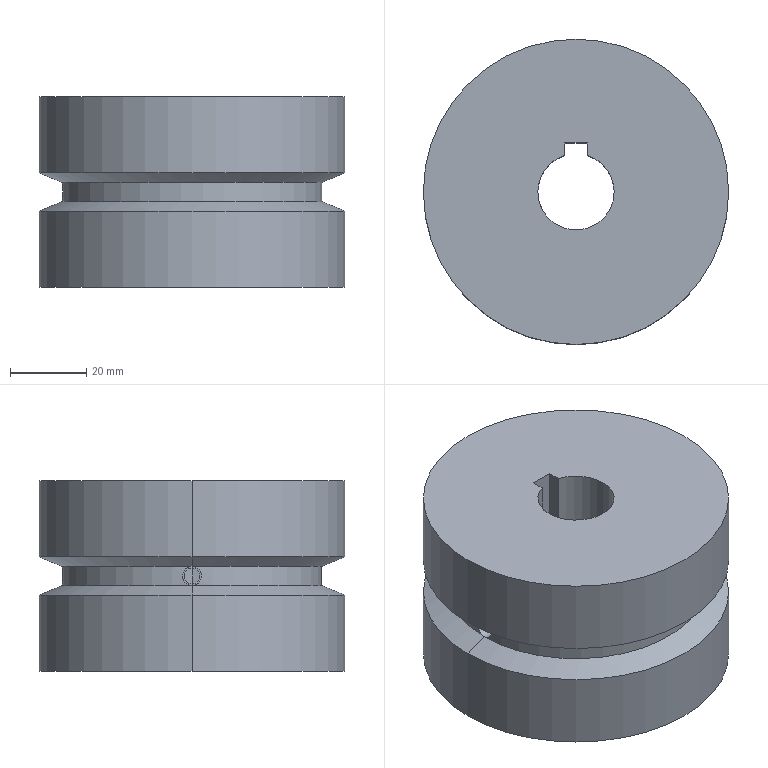Part | SolidWorks | features ICE 2, CirPattern 1, Extrusion 1, HoleWzd 1, RevCut 1 | 1 solid | 29 faces | box 80 x 80 x 50 mm | volume 223390 mm3 | cylinder 18 | plane 7 | cone 4 | commonest cylinder face diameters 4.2 x4 5 x4 80 x4 20 x3 68 x3
STEP:
#1=CARTESIAN_POINT('',(-20.,2.5,0.));
#2=VERTEX_POINT('',#1);
#3=CARTESIAN_POINT('',(-20.,-2.5,0.));
#4=VERTEX_POINT('',#3);
#5=CARTESIAN_POINT('',(-20.,0.,0.));
#6=DIRECTION('',(-1.,0.,0.));
#7=DIRECTION('',(0.,0.,1.));
#8=AXIS2_PLACEMENT_3D('',#5,#6,#7);
#9=CIRCLE('',#8,2.5);
#10=EDGE_CURVE('',#2,#4,#9,.T.);
#11=ORIENTED_EDGE('',*,*,#10,.F.);
#12=CARTESIAN_POINT('',(-33.908,2.5,0.));
#13=VERTEX_POINT('',#12);
#14=CARTESIAN_POINT('',(-20.,2.5,0.));
#15=DIRECTION('',(-1.,0.,0.));
#16=VECTOR('',#15,1000.);
#17=LINE('',#14,#16);
#18=EDGE_CURVE('',#2,#13,#17,.T.);
#19=ORIENTED_EDGE('',*,*,#18,.T.);
#20=CARTESIAN_POINT('',(-34.,0.,-2.5));
#21=VERTEX_POINT('',#20);
#22=CARTESIAN_POINT('',(-33.908,2.5,0.));
#23=CARTESIAN_POINT('',(-33.908,2.5,-0.1649));
#24=CARTESIAN_POINT('',(-33.909,2.484,-0.3277));
#25=CARTESIAN_POINT('',(-33.914,2.42,-0.6471));
#26=CARTESIAN_POINT('',(-33.917,2.372,-0.8056));
#27=CARTESIAN_POINT('',(-33.926,2.247,-1.108));
#28=CARTESIAN_POINT('',(-33.931,2.17,-1.252));
#29=CARTESIAN_POINT('',(-33.942,1.989,-1.523));
#30=CARTESIAN_POINT('',(-33.948,1.884,-1.652));
#31=CARTESIAN_POINT('',(-33.96,1.653,-1.883));
#32=CARTESIAN_POINT('',(-33.966,1.527,-1.986));
#33=CARTESIAN_POINT('',(-33.977,1.255,-2.169));
#34=CARTESIAN_POINT('',(-33.982,1.109,-2.246));
#35=CARTESIAN_POINT('',(-33.995,0.6583,-2.434));
#36=CARTESIAN_POINT('',(-34.,0.3302,-2.5));
#37=CARTESIAN_POINT('',(-34.,0.,-2.5));
#38=B_SPLINE_CURVE_WITH_KNOTS('',3,(#22,#23,#24,#25,#26,#27,#28,#29,#30,#31,#32,#33,#34,#35,#36,#37),.UNSPECIFIED.,.F.,.F.,(4,2,2,2,2,2,2,4),(0.01173,0.01222,0.01271,0.01319,0.01368,0.01417,0.01466,0.01564),.UNSPECIFIED.);
#39=EDGE_CURVE('',#13,#21,#38,.T.);
#40=ORIENTED_EDGE('',*,*,#39,.T.);
#41=CARTESIAN_POINT('',(-33.908,-2.5,0.));
#42=VERTEX_POINT('',#41);
#43=CARTESIAN_POINT('',(-34.,0.,-2.5));
#44=CARTESIAN_POINT('',(-34.,-0.1653,-2.5));
#45=CARTESIAN_POINT('',(-33.999,-0.3278,-2.484));
#46=CARTESIAN_POINT('',(-33.994,-0.6475,-2.42));
#47=CARTESIAN_POINT('',(-33.991,-0.8063,-2.372));
#48=CARTESIAN_POINT('',(-33.982,-1.109,-2.246));
#49=CARTESIAN_POINT('',(-33.977,-1.253,-2.17));
#50=CARTESIAN_POINT('',(-33.966,-1.525,-1.988));
#51=CARTESIAN_POINT('',(-33.96,-1.653,-1.882));
#52=CARTESIAN_POINT('',(-33.948,-1.884,-1.652));
#53=CARTESIAN_POINT('',(-33.942,-1.987,-1.526));
#54=CARTESIAN_POINT('',(-33.931,-2.17,-1.252));
#55=CARTESIAN_POINT('',(-33.926,-2.247,-1.107));
#56=CARTESIAN_POINT('',(-33.917,-2.372,-0.806));
#57=CARTESIAN_POINT('',(-33.914,-2.42,-0.6483));
#58=CARTESIAN_POINT('',(-33.909,-2.484,-0.3255));
#59=CARTESIAN_POINT('',(-33.908,-2.5,-0.1632));
#60=CARTESIAN_POINT('',(-33.908,-2.5,0.));
#61=B_SPLINE_CURVE_WITH_KNOTS('',3,(#43,#44,#45,#46,#47,#48,#49,#50,#51,#52,#53,#54,#55,#56,#57,#58,#59,#60),.UNSPECIFIED.,.F.,.F.,(4,2,2,2,2,2,2,2,4),(0.,0.0004888,0.0009776,0.001466,0.001955,0.002444,0.002933,0.003421,0.00391),.UNSPECIFIED.);
#62=EDGE_CURVE('',#21,#42,#61,.T.);
#63=ORIENTED_EDGE('',*,*,#62,.T.);
#64=CARTESIAN_POINT('',(-20.,-2.5,0.));
#65=DIRECTION('',(-1.,0.,0.));
#66=VECTOR('',#65,1000.);
#67=LINE('',#64,#66);
#68=EDGE_CURVE('',#4,#42,#67,.T.);
#69=ORIENTED_EDGE('',*,*,#68,.F.);
#70=EDGE_LOOP('',(#11,#19,#40,#63,#69));
#71=FACE_OUTER_BOUND('',#70,.T.);
#72=CARTESIAN_POINT('',(-20.,0.,0.));
#73=DIRECTION('',(-1.,0.,0.));
#74=DIRECTION('',(0.,-1.,0.));
#75=AXIS2_PLACEMENT_3D('',#72,#73,#74);
#76=CYLINDRICAL_SURFACE('',#75,2.5);
#77=ADVANCED_FACE('',(#71),#76,.F.);
#78=CARTESIAN_POINT('',(0.,20.,-2.5));
#79=VERTEX_POINT('',#78);
#80=CARTESIAN_POINT('',(0.,20.,2.5));
#81=VERTEX_POINT('',#80);
#82=CARTESIAN_POINT('',(0.,20.,0.));
#83=DIRECTION('',(0.,1.,0.));
#84=DIRECTION('',(0.,0.,1.));
#85=AXIS2_PLACEMENT_3D('',#82,#83,#84);
#86=CIRCLE('',#85,2.5);
#87=EDGE_CURVE('',#79,#81,#86,.T.);
#88=ORIENTED_EDGE('',*,*,#87,.F.);
#89=CARTESIAN_POINT('',(0.,34.,-2.5));
#90=VERTEX_POINT('',#89);
#91=CARTESIAN_POINT('',(0.,20.,-2.5));
#92=DIRECTION('',(0.,1.,0.));
#93=VECTOR('',#92,1000.);
#94=LINE('',#91,#93);
#95=EDGE_CURVE('',#79,#90,#94,.T.);
#96=ORIENTED_EDGE('',*,*,#95,.T.);
#97=CARTESIAN_POINT('',(0.,34.,2.5));
#98=VERTEX_POINT('',#97);
#99=CARTESIAN_POINT('',(0.,34.,-2.5));
#100=CARTESIAN_POINT('',(-0.1652,34.,-2.5));
#101=CARTESIAN_POINT('',(-0.3277,33.999,-2.484));
#102=CARTESIAN_POINT('',(-0.6473,33.994,-2.42));
#103=CARTESIAN_POINT('',(-0.8061,33.991,-2.372));
#104=CARTESIAN_POINT('',(-1.109,33.982,-2.247));
#105=CARTESIAN_POINT('',(-1.252,33.977,-2.17));
#106=CARTESIAN_POINT('',(-1.524,33.966,-1.988));
#107=CARTESIAN_POINT('',(-1.653,33.96,-1.883));
#108=CARTESIAN_POINT('',(-1.883,33.948,-1.652));
#109=CARTESIAN_POINT('',(-1.987,33.942,-1.526));
#110=CARTESIAN_POINT('',(-2.17,33.931,-1.253));
#111=CARTESIAN_POINT('',(-2.247,33.926,-1.108));
#112=CARTESIAN_POINT('',(-2.372,33.917,-0.8067));
#113=CARTESIAN_POINT('',(-2.42,33.914,-0.649));
#114=CARTESIAN_POINT('',(-2.484,33.909,-0.3263));
#115=CARTESIAN_POINT('',(-2.5,33.908,-0.164));
#116=CARTESIAN_POINT('',(-2.5,33.908,0.1622));
#117=CARTESIAN_POINT('',(-2.484,33.909,0.3279));
#118=CARTESIAN_POINT('',(-2.42,33.914,0.6486));
#119=CARTESIAN_POINT('',(-2.373,33.917,0.8045));
#120=CARTESIAN_POINT('',(-2.247,33.926,1.107));
#121=CARTESIAN_POINT('',(-2.169,33.931,1.254));
#122=CARTESIAN_POINT('',(-1.988,33.942,1.524));
#123=CARTESIAN_POINT('',(-1.885,33.948,1.651));
#124=CARTESIAN_POINT('',(-1.651,33.96,1.884));
#125=CARTESIAN_POINT('',(-1.525,33.966,1.988));
#126=CARTESIAN_POINT('',(-1.254,33.977,2.169));
#127=CARTESIAN_POINT('',(-1.108,33.982,2.247));
#128=CARTESIAN_POINT('',(-0.8053,33.991,2.372));
#129=CARTESIAN_POINT('',(-0.6494,33.994,2.42));
#130=CARTESIAN_POINT('',(-0.3289,33.999,2.484));
#131=CARTESIAN_POINT('',(-0.1632,34.,2.5));
#132=CARTESIAN_POINT('',(0.,34.,2.5));
#133=B_SPLINE_CURVE_WITH_KNOTS('',3,(#99,#100,#101,#102,#103,#104,#105,#106,#107,#108,#109,#110,#111,#112,#113,#114,#115,#116,#117,#118,#119,#120,#121,#122,#123,#124,#125,#126,#127,#128,#129,#130,#131,#132),.UNSPECIFIED.,.F.,.F.,(4,2,2,2,2,2,2,2,2,2,2,2,2,2,2,2,4),(0.,0.0004887,0.0009773,0.001466,0.001955,0.002443,0.002932,0.003421,0.003909,0.004398,0.004887,0.005375,0.005864,0.006353,0.006841,0.00733,0.007819),.UNSPECIFIED.);
#134=EDGE_CURVE('',#90,#98,#133,.T.);
#135=ORIENTED_EDGE('',*,*,#134,.T.);
#136=CARTESIAN_POINT('',(0.,20.,2.5));
#137=DIRECTION('',(0.,1.,0.));
#138=VECTOR('',#137,1000.);
#139=LINE('',#136,#138);
#140=EDGE_CURVE('',#81,#98,#139,.T.);
#141=ORIENTED_EDGE('',*,*,#140,.F.);
#142=EDGE_LOOP('',(#88,#96,#135,#141));
#143=FACE_OUTER_BOUND('',#142,.T.);
#144=CARTESIAN_POINT('',(0.,20.,0.));
#145=DIRECTION('',(0.,1.,0.));
#146=DIRECTION('',(0.,0.,1.));
#147=AXIS2_PLACEMENT_3D('',#144,#145,#146);
#148=CYLINDRICAL_SURFACE('',#147,2.5);
#149=ADVANCED_FACE('',(#143),#148,.F.);
#150=CARTESIAN_POINT('',(34.,0.,-2.5));
#151=VERTEX_POINT('',#150);
#152=CARTESIAN_POINT('',(0.,0.,-2.5));
#153=DIRECTION('',(0.,0.,1.));
#154=DIRECTION('',(1.,0.,0.));
#155=AXIS2_PLACEMENT_3D('',#152,#153,#154);
#156=CIRCLE('',#155,34.);
#157=EDGE_CURVE('',#151,#90,#156,.T.);
#158=ORIENTED_EDGE('',*,*,#157,.F.);
#159=CARTESIAN_POINT('',(40.,0.,-5.));
#160=VERTEX_POINT('',#159);
#161=CARTESIAN_POINT('',(34.,0.,-2.5));
#162=DIRECTION('',(0.9231,0.,-0.3846));
#163=VECTOR('',#162,1000.);
#164=LINE('',#161,#163);
#165=EDGE_CURVE('',#151,#160,#164,.T.);
#166=ORIENTED_EDGE('',*,*,#165,.T.);
#167=CARTESIAN_POINT('',(-40.,0.,-5.));
#168=VERTEX_POINT('',#167);
#169=CARTESIAN_POINT('',(0.,0.,-5.));
#170=DIRECTION('',(0.,0.,1.));
#171=DIRECTION('',(1.,0.,0.));
#172=AXIS2_PLACEMENT_3D('',#169,#170,#171);
#173=CIRCLE('',#172,40.);
#174=EDGE_CURVE('',#160,#168,#173,.T.);
#175=ORIENTED_EDGE('',*,*,#174,.T.);
#176=CARTESIAN_POINT('',(-34.,0.,-2.5));
#177=DIRECTION('',(-0.9231,0.,-0.3846));
#178=VECTOR('',#177,1000.);
#179=LINE('',#176,#178);
#180=EDGE_CURVE('',#21,#168,#179,.T.);
#181=ORIENTED_EDGE('',*,*,#180,.F.);
#182=CARTESIAN_POINT('',(0.,0.,-2.5));
#183=DIRECTION('',(0.,0.,1.));
#184=DIRECTION('',(1.,0.,0.));
#185=AXIS2_PLACEMENT_3D('',#182,#183,#184);
#186=CIRCLE('',#185,34.);
#187=EDGE_CURVE('',#90,#21,#186,.T.);
#188=ORIENTED_EDGE('',*,*,#187,.F.);
#189=EDGE_LOOP('',(#158,#166,#175,#181,#188));
#190=FACE_OUTER_BOUND('',#189,.T.);
#191=CARTESIAN_POINT('',(0.,0.,-2.5));
#192=DIRECTION('',(0.,0.,-1.));
#193=DIRECTION('',(-1.,0.,0.));
#194=AXIS2_PLACEMENT_3D('',#191,#192,#193);
#195=CONICAL_SURFACE('',#194,34.,1.176);
#196=ADVANCED_FACE('',(#190),#195,.T.);
#197=CARTESIAN_POINT('',(-34.,0.,2.5));
#198=VERTEX_POINT('',#197);
#199=CARTESIAN_POINT('',(0.,0.,2.5));
#200=DIRECTION('',(0.,0.,1.));
#201=DIRECTION('',(1.,0.,0.));
#202=AXIS2_PLACEMENT_3D('',#199,#200,#201);
#203=CIRCLE('',#202,34.);
#204=EDGE_CURVE('',#98,#198,#203,.T.);
#205=ORIENTED_EDGE('',*,*,#204,.T.);
#206=CARTESIAN_POINT('',(-40.,0.,5.));
#207=VERTEX_POINT('',#206);
#208=CARTESIAN_POINT('',(-40.,0.,5.));
#209=DIRECTION('',(-0.9231,0.,0.3846));
#210=VECTOR('',#209,1000.);
#211=LINE('',#208,#210);
#212=EDGE_CURVE('',#198,#207,#211,.T.);
#213=ORIENTED_EDGE('',*,*,#212,.T.);
#214=CARTESIAN_POINT('',(40.,0.,5.));
#215=VERTEX_POINT('',#214);
#216=CARTESIAN_POINT('',(0.,0.,5.));
#217=DIRECTION('',(0.,0.,1.));
#218=DIRECTION('',(1.,0.,0.));
#219=AXIS2_PLACEMENT_3D('',#216,#217,#218);
#220=CIRCLE('',#219,40.);
#221=EDGE_CURVE('',#215,#207,#220,.T.);
#222=ORIENTED_EDGE('',*,*,#221,.F.);
#223=CARTESIAN_POINT('',(34.,0.,2.5));
#224=VERTEX_POINT('',#223);
#225=CARTESIAN_POINT('',(40.,0.,5.));
#226=DIRECTION('',(0.9231,0.,0.3846));
#227=VECTOR('',#226,1000.);
#228=LINE('',#225,#227);
#229=EDGE_CURVE('',#224,#215,#228,.T.);
#230=ORIENTED_EDGE('',*,*,#229,.F.);
#231=CARTESIAN_POINT('',(0.,0.,2.5));
#232=DIRECTION('',(0.,0.,1.));
#233=DIRECTION('',(1.,0.,0.));
#234=AXIS2_PLACEMENT_3D('',#231,#232,#233);
#235=CIRCLE('',#234,34.);
#236=EDGE_CURVE('',#224,#98,#235,.T.);
#237=ORIENTED_EDGE('',*,*,#236,.T.);
#238=EDGE_LOOP('',(#205,#213,#222,#230,#237));
#239=FACE_OUTER_BOUND('',#238,.T.);
#240=CARTESIAN_POINT('',(0.,0.,5.));
#241=DIRECTION('',(0.,0.,1.));
#242=DIRECTION('',(1.,0.,0.));
#243=AXIS2_PLACEMENT_3D('',#240,#241,#242);
#244=CONICAL_SURFACE('',#243,40.,1.176);
#245=ADVANCED_FACE('',(#239),#244,.T.);
#246=CARTESIAN_POINT('',(-10.,0.,25.));
#247=VERTEX_POINT('',#246);
#248=CARTESIAN_POINT('',(10.,0.,25.));
#249=VERTEX_POINT('',#248);
#250=CARTESIAN_POINT('',(0.,0.,25.));
#251=DIRECTION('',(0.,0.,1.));
#252=DIRECTION('',(1.,0.,0.));
#253=AXIS2_PLACEMENT_3D('',#250,#251,#252);
#254=CIRCLE('',#253,10.);
#255=EDGE_CURVE('',#247,#249,#254,.T.);
#256=ORIENTED_EDGE('',*,*,#255,.T.);
#257=CARTESIAN_POINT('',(10.,0.,-25.));
#258=VERTEX_POINT('',#257);
#259=CARTESIAN_POINT('',(10.,0.,25.));
#260=DIRECTION('',(0.,0.,-1.));
#261=VECTOR('',#260,1000.);
#262=LINE('',#259,#261);
#263=EDGE_CURVE('',#249,#258,#262,.T.);
#264=ORIENTED_EDGE('',*,*,#263,.T.);
#265=CARTESIAN_POINT('',(-10.,0.,-25.));
#266=VERTEX_POINT('',#265);
#267=CARTESIAN_POINT('',(0.,0.,-25.));
#268=DIRECTION('',(0.,0.,1.));
#269=DIRECTION('',(1.,0.,0.));
#270=AXIS2_PLACEMENT_3D('',#267,#268,#269);
#271=CIRCLE('',#270,10.);
#272=EDGE_CURVE('',#266,#258,#271,.T.);
#273=ORIENTED_EDGE('',*,*,#272,.F.);
#274=CARTESIAN_POINT('',(-10.,0.,-2.1));
#275=VERTEX_POINT('',#274);
#276=CARTESIAN_POINT('',(-10.,0.,25.));
#277=DIRECTION('',(0.,0.,-1.));
#278=VECTOR('',#277,1000.);
#279=LINE('',#276,#278);
#280=EDGE_CURVE('',#275,#266,#279,.T.);
#281=ORIENTED_EDGE('',*,*,#280,.F.);
#282=CARTESIAN_POINT('',(-10.,0.,2.1));
#283=VERTEX_POINT('',#282);
#284=CARTESIAN_POINT('',(-10.,0.,2.1));
#285=CARTESIAN_POINT('',(-10.,-0.2745,2.1));
#286=CARTESIAN_POINT('',(-9.988,-0.5515,2.045));
#287=CARTESIAN_POINT('',(-9.957,-0.9307,1.887));
#288=CARTESIAN_POINT('',(-9.945,-1.053,1.822));
#289=CARTESIAN_POINT('',(-9.918,-1.282,1.669));
#290=CARTESIAN_POINT('',(-9.904,-1.387,1.582));
#291=CARTESIAN_POINT('',(-9.875,-1.581,1.389));
#292=CARTESIAN_POINT('',(-9.86,-1.669,1.281));
#293=CARTESIAN_POINT('',(-9.833,-1.821,1.054));
#294=CARTESIAN_POINT('',(-9.821,-1.886,0.9337));
#295=CARTESIAN_POINT('',(-9.789,-2.045,0.5514));
#296=CARTESIAN_POINT('',(-9.777,-2.1,0.2782));
#297=CARTESIAN_POINT('',(-9.777,-2.1,-0.1376));
#298=CARTESIAN_POINT('',(-9.78,-2.087,-0.2742));
#299=CARTESIAN_POINT('',(-9.791,-2.033,-0.5435));
#300=CARTESIAN_POINT('',(-9.8,-1.992,-0.6774));
#301=CARTESIAN_POINT('',(-9.82,-1.887,-0.931));
#302=CARTESIAN_POINT('',(-9.833,-1.823,-1.052));
#303=CARTESIAN_POINT('',(-9.86,-1.67,-1.28));
#304=CARTESIAN_POINT('',(-9.875,-1.582,-1.387));
#305=CARTESIAN_POINT('',(-9.918,-1.293,-1.677));
#306=CARTESIAN_POINT('',(-9.947,-1.06,-1.834));
#307=CARTESIAN_POINT('',(-9.978,-0.6807,-1.991));
#308=CARTESIAN_POINT('',(-9.986,-0.5474,-2.032));
#309=CARTESIAN_POINT('',(-9.997,-0.2764,-2.086));
#310=CARTESIAN_POINT('',(-10.,-0.1391,-2.1));
#311=CARTESIAN_POINT('',(-10.,0.,-2.1));
#312=B_SPLINE_CURVE_WITH_KNOTS('',3,(#284,#285,#286,#287,#288,#289,#290,#291,#292,#293,#294,#295,#296,#297,#298,#299,#300,#301,#302,#303,#304,#305,#306,#307,#308,#309,#310,#311),.UNSPECIFIED.,.F.,.F.,(4,2,2,2,2,2,2,2,2,2,2,2,2,4),(0.006584,0.007407,0.007818,0.008229,0.008641,0.009052,0.009875,0.01029,0.0107,0.01111,0.01152,0.01234,0.01275,0.01317),.UNSPECIFIED.);
#313=EDGE_CURVE('',#283,#275,#312,.T.);
#314=ORIENTED_EDGE('',*,*,#313,.F.);
#315=CARTESIAN_POINT('',(-10.,0.,25.));
#316=DIRECTION('',(0.,0.,-1.));
#317=VECTOR('',#316,1000.);
#318=LINE('',#315,#317);
#319=EDGE_CURVE('',#247,#283,#318,.T.);
#320=ORIENTED_EDGE('',*,*,#319,.F.);
#321=EDGE_LOOP('',(#256,#264,#273,#281,#314,#320));
#322=FACE_OUTER_BOUND('',#321,.T.);
#323=CARTESIAN_POINT('',(0.,0.,25.));
#324=DIRECTION('',(0.,0.,-1.));
#325=DIRECTION('',(-1.,0.,0.));
#326=AXIS2_PLACEMENT_3D('',#323,#324,#325);
#327=CYLINDRICAL_SURFACE('',#326,10.);
#328=ADVANCED_FACE('',(#322),#327,.F.);
#329=CARTESIAN_POINT('',(-3.,9.539,25.));
#330=VERTEX_POINT('',#329);
#331=CARTESIAN_POINT('',(0.,0.,25.));
#332=DIRECTION('',(0.,0.,1.));
#333=DIRECTION('',(1.,0.,0.));
#334=AXIS2_PLACEMENT_3D('',#331,#332,#333);
#335=CIRCLE('',#334,10.);
#336=EDGE_CURVE('',#330,#247,#335,.T.);
#337=ORIENTED_EDGE('',*,*,#336,.T.);
#338=ORIENTED_EDGE('',*,*,#319,.T.);
#339=CARTESIAN_POINT('',(-10.,0.,-2.1));
#340=CARTESIAN_POINT('',(-10.,0.1392,-2.1));
#341=CARTESIAN_POINT('',(-9.997,0.2759,-2.086));
#342=CARTESIAN_POINT('',(-9.986,0.5449,-2.033));
#343=CARTESIAN_POINT('',(-9.978,0.6785,-1.992));
#344=CARTESIAN_POINT('',(-9.957,0.9326,-1.887));
#345=CARTESIAN_POINT('',(-9.945,1.053,-1.822));
#346=CARTESIAN_POINT('',(-9.918,1.281,-1.67));
#347=CARTESIAN_POINT('',(-9.904,1.389,-1.581));
#348=CARTESIAN_POINT('',(-9.86,1.678,-1.291));
#349=CARTESIAN_POINT('',(-9.831,1.835,-1.058));
#350=CARTESIAN_POINT('',(-9.8,1.992,-0.6788));
#351=CARTESIAN_POINT('',(-9.791,2.032,-0.546));
#352=CARTESIAN_POINT('',(-9.78,2.087,-0.2748));
#353=CARTESIAN_POINT('',(-9.777,2.1,-0.1382));
#354=CARTESIAN_POINT('',(-9.777,2.1,0.1366));
#355=CARTESIAN_POINT('',(-9.78,2.086,0.2762));
#356=CARTESIAN_POINT('',(-9.791,2.032,0.5458));
#357=CARTESIAN_POINT('',(-9.8,1.993,0.6769));
#358=CARTESIAN_POINT('',(-9.831,1.834,1.059));
#359=CARTESIAN_POINT('',(-9.86,1.68,1.29));
#360=CARTESIAN_POINT('',(-9.904,1.387,1.583));
#361=CARTESIAN_POINT('',(-9.918,1.282,1.669));
#362=CARTESIAN_POINT('',(-9.945,1.054,1.821));
#363=CARTESIAN_POINT('',(-9.957,0.9314,1.887));
#364=CARTESIAN_POINT('',(-9.978,0.6776,1.992));
#365=CARTESIAN_POINT('',(-9.986,0.5467,2.032));
#366=CARTESIAN_POINT('',(-9.997,0.2767,2.086));
#367=CARTESIAN_POINT('',(-10.,0.1373,2.1));
#368=CARTESIAN_POINT('',(-10.,0.,2.1));
#369=B_SPLINE_CURVE_WITH_KNOTS('',3,(#339,#340,#341,#342,#343,#344,#345,#346,#347,#348,#349,#350,#351,#352,#353,#354,#355,#356,#357,#358,#359,#360,#361,#362,#363,#364,#365,#366,#367,#368),.UNSPECIFIED.,.F.,.F.,(4,2,2,2,2,2,2,2,2,2,2,2,2,2,4),(0.,0.0004115,0.000823,0.001234,0.001646,0.002469,0.00288,0.003292,0.003703,0.004115,0.004938,0.005349,0.005761,0.006172,0.006584),.UNSPECIFIED.);
#370=EDGE_CURVE('',#275,#283,#369,.T.);
#371=ORIENTED_EDGE('',*,*,#370,.F.);
#372=ORIENTED_EDGE('',*,*,#280,.T.);
#373=CARTESIAN_POINT('',(-3.,9.539,-25.));
#374=VERTEX_POINT('',#373);
#375=CARTESIAN_POINT('',(0.,0.,-25.));
#376=DIRECTION('',(0.,0.,1.));
#377=DIRECTION('',(1.,0.,0.));
#378=AXIS2_PLACEMENT_3D('',#375,#376,#377);
#379=CIRCLE('',#378,10.);
#380=EDGE_CURVE('',#374,#266,#379,.T.);
#381=ORIENTED_EDGE('',*,*,#380,.F.);
#382=CARTESIAN_POINT('',(-3.,9.539,25.));
#383=DIRECTION('',(0.,0.,-1.));
#384=VECTOR('',#383,1000.);
#385=LINE('',#382,#384);
#386=EDGE_CURVE('',#330,#374,#385,.T.);
#387=ORIENTED_EDGE('',*,*,#386,.F.);
#388=EDGE_LOOP('',(#337,#338,#371,#372,#381,#387));
#389=FACE_OUTER_BOUND('',#388,.T.);
#390=CARTESIAN_POINT('',(0.,0.,25.));
#391=DIRECTION('',(0.,0.,-1.));
#392=DIRECTION('',(-1.,0.,0.));
#393=AXIS2_PLACEMENT_3D('',#390,#391,#392);
#394=CYLINDRICAL_SURFACE('',#393,10.);
#395=ADVANCED_FACE('',(#389),#394,.F.);
#396=ORIENTED_EDGE('',*,*,#174,.F.);
#397=CARTESIAN_POINT('',(40.,0.,-25.));
#398=VERTEX_POINT('',#397);
#399=CARTESIAN_POINT('',(40.,0.,25.));
#400=DIRECTION('',(0.,0.,-1.));
#401=VECTOR('',#400,1000.);
#402=LINE('',#399,#401);
#403=EDGE_CURVE('',#160,#398,#402,.T.);
#404=ORIENTED_EDGE('',*,*,#403,.T.);
#405=CARTESIAN_POINT('',(-40.,0.,-25.));
#406=VERTEX_POINT('',#405);
#407=CARTESIAN_POINT('',(0.,0.,-25.));
#408=DIRECTION('',(0.,0.,1.));
#409=DIRECTION('',(1.,0.,0.));
#410=AXIS2_PLACEMENT_3D('',#407,#408,#409);
#411=CIRCLE('',#410,40.);
#412=EDGE_CURVE('',#398,#406,#411,.T.);
#413=ORIENTED_EDGE('',*,*,#412,.T.);
#414=CARTESIAN_POINT('',(-40.,0.,25.));
#415=DIRECTION('',(0.,0.,-1.));
#416=VECTOR('',#415,1000.);
#417=LINE('',#414,#416);
#418=EDGE_CURVE('',#168,#406,#417,.T.);
#419=ORIENTED_EDGE('',*,*,#418,.F.);
#420=EDGE_LOOP('',(#396,#404,#413,#419));
#421=FACE_OUTER_BOUND('',#420,.T.);
#422=CARTESIAN_POINT('',(0.,0.,25.));
#423=DIRECTION('',(0.,0.,-1.));
#424=DIRECTION('',(-1.,0.,0.));
#425=AXIS2_PLACEMENT_3D('',#422,#423,#424);
#426=CYLINDRICAL_SURFACE('',#425,40.);
#427=ADVANCED_FACE('',(#421),#426,.T.);
#428=CARTESIAN_POINT('',(40.,0.,25.));
#429=VERTEX_POINT('',#428);
#430=CARTESIAN_POINT('',(-40.,0.,25.));
#431=VERTEX_POINT('',#430);
#432=CARTESIAN_POINT('',(0.,0.,25.));
#433=DIRECTION('',(0.,0.,1.));
#434=DIRECTION('',(1.,0.,0.));
#435=AXIS2_PLACEMENT_3D('',#432,#433,#434);
#436=CIRCLE('',#435,40.);
#437=EDGE_CURVE('',#429,#431,#436,.T.);
#438=ORIENTED_EDGE('',*,*,#437,.F.);
#439=CARTESIAN_POINT('',(40.,0.,25.));
#440=DIRECTION('',(0.,0.,-1.));
#441=VECTOR('',#440,1000.);
#442=LINE('',#439,#441);
#443=EDGE_CURVE('',#429,#215,#442,.T.);
#444=ORIENTED_EDGE('',*,*,#443,.T.);
#445=ORIENTED_EDGE('',*,*,#221,.T.);
#446=CARTESIAN_POINT('',(-40.,0.,25.));
#447=DIRECTION('',(0.,0.,-1.));
#448=VECTOR('',#447,1000.);
#449=LINE('',#446,#448);
#450=EDGE_CURVE('',#431,#207,#449,.T.);
#451=ORIENTED_EDGE('',*,*,#450,.F.);
#452=EDGE_LOOP('',(#438,#444,#445,#451));
#453=FACE_OUTER_BOUND('',#452,.T.);
#454=CARTESIAN_POINT('',(0.,0.,25.));
#455=DIRECTION('',(0.,0.,-1.));
#456=DIRECTION('',(-1.,0.,0.));
#457=AXIS2_PLACEMENT_3D('',#454,#455,#456);
#458=CYLINDRICAL_SURFACE('',#457,40.);
#459=ADVANCED_FACE('',(#453),#458,.T.);
#460=CARTESIAN_POINT('',(0.,20.,2.1));
#461=VERTEX_POINT('',#460);
#462=CARTESIAN_POINT('',(0.,20.,-2.1));
#463=VERTEX_POINT('',#462);
#464=CARTESIAN_POINT('',(0.,20.,0.));
#465=DIRECTION('',(0.,-1.,0.));
#466=DIRECTION('',(0.,0.,1.));
#467=AXIS2_PLACEMENT_3D('',#464,#465,#466);
#468=CIRCLE('',#467,2.1);
#469=EDGE_CURVE('',#461,#463,#468,.T.);
#470=ORIENTED_EDGE('',*,*,#469,.F.);
#471=CARTESIAN_POINT('',(0.,12.8,2.1));
#472=VERTEX_POINT('',#471);
#473=CARTESIAN_POINT('',(0.,0.,2.1));
#474=DIRECTION('',(0.,-1.,0.));
#475=VECTOR('',#474,1000.);
#476=LINE('',#473,#475);
#477=EDGE_CURVE('',#461,#472,#476,.T.);
#478=ORIENTED_EDGE('',*,*,#477,.T.);
#479=CARTESIAN_POINT('',(0.,12.8,-2.1));
#480=VERTEX_POINT('',#479);
#481=CARTESIAN_POINT('',(0.,12.8,0.));
#482=DIRECTION('',(0.,1.,0.));
#483=DIRECTION('',(0.,0.,1.));
#484=AXIS2_PLACEMENT_3D('',#481,#482,#483);
#485=CIRCLE('',#484,2.1);
#486=EDGE_CURVE('',#480,#472,#485,.T.);
#487=ORIENTED_EDGE('',*,*,#486,.F.);
#488=CARTESIAN_POINT('',(0.,0.,-2.1));
#489=DIRECTION('',(0.,-1.,0.));
#490=VECTOR('',#489,1000.);
#491=LINE('',#488,#490);
#492=EDGE_CURVE('',#463,#480,#491,.T.);
#493=ORIENTED_EDGE('',*,*,#492,.F.);
#494=EDGE_LOOP('',(#470,#478,#487,#493));
#495=FACE_OUTER_BOUND('',#494,.T.);
#496=CARTESIAN_POINT('',(0.,0.,0.));
#497=DIRECTION('',(0.,-1.,0.));
#498=DIRECTION('',(0.,0.,-1.));
#499=AXIS2_PLACEMENT_3D('',#496,#497,#498);
#500=CYLINDRICAL_SURFACE('',#499,2.1);
#501=ADVANCED_FACE('',(#495),#500,.F.);
#502=CARTESIAN_POINT('',(-20.,0.,2.1));
#503=VERTEX_POINT('',#502);
#504=CARTESIAN_POINT('',(-20.,0.,-2.1));
#505=VERTEX_POINT('',#504);
#506=CARTESIAN_POINT('',(-20.,0.,0.));
#507=DIRECTION('',(1.,0.,0.));
#508=DIRECTION('',(0.,-1.,0.));
#509=AXIS2_PLACEMENT_3D('',#506,#507,#508);
#510=CIRCLE('',#509,2.1);
#511=EDGE_CURVE('',#503,#505,#510,.T.);
#512=ORIENTED_EDGE('',*,*,#511,.F.);
#513=CARTESIAN_POINT('',(0.,0.,2.1));
#514=DIRECTION('',(1.,0.,0.));
#515=VECTOR('',#514,1000.);
#516=LINE('',#513,#515);
#517=EDGE_CURVE('',#503,#283,#516,.T.);
#518=ORIENTED_EDGE('',*,*,#517,.T.);
#519=ORIENTED_EDGE('',*,*,#313,.T.);
#520=CARTESIAN_POINT('',(0.,0.,-2.1));
#521=DIRECTION('',(1.,0.,0.));
#522=VECTOR('',#521,1000.);
#523=LINE('',#520,#522);
#524=EDGE_CURVE('',#505,#275,#523,.T.);
#525=ORIENTED_EDGE('',*,*,#524,.F.);
#526=EDGE_LOOP('',(#512,#518,#519,#525));
#527=FACE_OUTER_BOUND('',#526,.T.);
#528=CARTESIAN_POINT('',(0.,0.,0.));
#529=DIRECTION('',(1.,0.,0.));
#530=DIRECTION('',(0.,0.,-1.));
#531=AXIS2_PLACEMENT_3D('',#528,#529,#530);
#532=CYLINDRICAL_SURFACE('',#531,2.1);
#533=ADVANCED_FACE('',(#527),#532,.F.);
#534=CARTESIAN_POINT('',(0.,0.,-2.5));
#535=DIRECTION('',(0.,0.,1.));
#536=DIRECTION('',(1.,0.,0.));
#537=AXIS2_PLACEMENT_3D('',#534,#535,#536);
#538=CIRCLE('',#537,34.);
#539=EDGE_CURVE('',#21,#151,#538,.T.);
#540=ORIENTED_EDGE('',*,*,#539,.T.);
#541=CARTESIAN_POINT('',(34.,0.,0.));
#542=DIRECTION('',(0.,0.,1.));
#543=VECTOR('',#542,1000.);
#544=LINE('',#541,#543);
#545=EDGE_CURVE('',#151,#224,#544,.T.);
#546=ORIENTED_EDGE('',*,*,#545,.T.);
#547=CARTESIAN_POINT('',(0.,0.,2.5));
#548=DIRECTION('',(0.,0.,1.));
#549=DIRECTION('',(1.,0.,0.));
#550=AXIS2_PLACEMENT_3D('',#547,#548,#549);
#551=CIRCLE('',#550,34.);
#552=EDGE_CURVE('',#198,#224,#551,.T.);
#553=ORIENTED_EDGE('',*,*,#552,.F.);
#554=CARTESIAN_POINT('',(-33.908,-2.5,0.));
#555=CARTESIAN_POINT('',(-33.908,-2.5,0.1631));
#556=CARTESIAN_POINT('',(-33.909,-2.484,0.3287));
#557=CARTESIAN_POINT('',(-33.914,-2.42,0.6493));
#558=CARTESIAN_POINT('',(-33.917,-2.372,0.8051));
#559=CARTESIAN_POINT('',(-33.926,-2.247,1.108));
#560=CARTESIAN_POINT('',(-33.931,-2.169,1.254));
#561=CARTESIAN_POINT('',(-33.942,-1.988,1.525));
#562=CARTESIAN_POINT('',(-33.948,-1.884,1.651));
#563=CARTESIAN_POINT('',(-33.96,-1.651,1.884));
#564=CARTESIAN_POINT('',(-33.966,-1.525,1.988));
#565=CARTESIAN_POINT('',(-33.977,-1.254,2.169));
#566=CARTESIAN_POINT('',(-33.982,-1.108,2.247));
#567=CARTESIAN_POINT('',(-33.991,-0.8051,2.372));
#568=CARTESIAN_POINT('',(-33.994,-0.6493,2.42));
#569=CARTESIAN_POINT('',(-33.999,-0.3289,2.484));
#570=CARTESIAN_POINT('',(-34.,-0.1632,2.5));
#571=CARTESIAN_POINT('',(-34.,0.,2.5));
#572=B_SPLINE_CURVE_WITH_KNOTS('',3,(#554,#555,#556,#557,#558,#559,#560,#561,#562,#563,#564,#565,#566,#567,#568,#569,#570,#571),.UNSPECIFIED.,.F.,.F.,(4,2,2,2,2,2,2,2,4),(0.00391,0.004399,0.004887,0.005376,0.005865,0.006353,0.006842,0.00733,0.007819),.UNSPECIFIED.);
#573=EDGE_CURVE('',#42,#198,#572,.T.);
#574=ORIENTED_EDGE('',*,*,#573,.F.);
#575=ORIENTED_EDGE('',*,*,#62,.F.);
#576=EDGE_LOOP('',(#540,#546,#553,#574,#575));
#577=FACE_OUTER_BOUND('',#576,.T.);
#578=CARTESIAN_POINT('',(0.,0.,0.));
#579=DIRECTION('',(0.,0.,1.));
#580=DIRECTION('',(1.,0.,0.));
#581=AXIS2_PLACEMENT_3D('',#578,#579,#580);
#582=CYLINDRICAL_SURFACE('',#581,34.);
#583=ADVANCED_FACE('',(#577),#582,.T.);
#584=ORIENTED_EDGE('',*,*,#545,.F.);
#585=ORIENTED_EDGE('',*,*,#157,.T.);
#586=CARTESIAN_POINT('',(0.,34.,2.5));
#587=CARTESIAN_POINT('',(0.1632,34.,2.5));
#588=CARTESIAN_POINT('',(0.3253,33.999,2.484));
#589=CARTESIAN_POINT('',(0.6477,33.994,2.42));
#590=CARTESIAN_POINT('',(0.8057,33.991,2.372));
#591=CARTESIAN_POINT('',(1.257,33.978,2.185));
#592=CARTESIAN_POINT('',(1.536,33.966,1.999));
#593=CARTESIAN_POINT('',(1.882,33.948,1.654));
#594=CARTESIAN_POINT('',(1.987,33.942,1.525));
#595=CARTESIAN_POINT('',(2.169,33.931,1.254));
#596=CARTESIAN_POINT('',(2.246,33.926,1.11));
#597=CARTESIAN_POINT('',(2.372,33.917,0.8078));
#598=CARTESIAN_POINT('',(2.42,33.914,0.6489));
#599=CARTESIAN_POINT('',(2.484,33.909,0.3293));
#600=CARTESIAN_POINT('',(2.5,33.908,0.167));
#601=CARTESIAN_POINT('',(2.5,33.908,-0.163));
#602=CARTESIAN_POINT('',(2.484,33.909,-0.3259));
#603=CARTESIAN_POINT('',(2.421,33.914,-0.6455));
#604=CARTESIAN_POINT('',(2.373,33.917,-0.8041));
#605=CARTESIAN_POINT('',(2.247,33.926,-1.107));
#606=CARTESIAN_POINT('',(2.171,33.931,-1.251));
#607=CARTESIAN_POINT('',(1.99,33.942,-1.522));
#608=CARTESIAN_POINT('',(1.884,33.948,-1.651));
#609=CARTESIAN_POINT('',(1.654,33.96,-1.882));
#610=CARTESIAN_POINT('',(1.528,33.966,-1.985));
#611=CARTESIAN_POINT('',(1.255,33.977,-2.168));
#612=CARTESIAN_POINT('',(1.11,33.982,-2.246));
#613=CARTESIAN_POINT('',(0.6587,33.995,-2.434));
#614=CARTESIAN_POINT('',(0.3304,34.,-2.5));
#615=CARTESIAN_POINT('',(0.,34.,-2.5));
#616=B_SPLINE_CURVE_WITH_KNOTS('',3,(#586,#587,#588,#589,#590,#591,#592,#593,#594,#595,#596,#597,#598,#599,#600,#601,#602,#603,#604,#605,#606,#607,#608,#609,#610,#611,#612,#613,#614,#615),.UNSPECIFIED.,.F.,.F.,(4,2,2,2,2,2,2,2,2,2,2,2,2,2,4),(0.007819,0.008307,0.008796,0.009773,0.01026,0.01075,0.01124,0.01173,0.01222,0.0127,0.01319,0.01368,0.01417,0.01466,0.01564),.UNSPECIFIED.);
#617=EDGE_CURVE('',#98,#90,#616,.T.);
#618=ORIENTED_EDGE('',*,*,#617,.F.);
#619=ORIENTED_EDGE('',*,*,#236,.F.);
#620=EDGE_LOOP('',(#584,#585,#618,#619));
#621=FACE_OUTER_BOUND('',#620,.T.);
#622=CARTESIAN_POINT('',(0.,0.,0.));
#623=DIRECTION('',(0.,0.,1.));
#624=DIRECTION('',(1.,0.,0.));
#625=AXIS2_PLACEMENT_3D('',#622,#623,#624);
#626=CYLINDRICAL_SURFACE('',#625,34.);
#627=ADVANCED_FACE('',(#621),#626,.T.);
#628=ORIENTED_EDGE('',*,*,#517,.F.);
#629=CARTESIAN_POINT('',(-20.,0.,0.));
#630=DIRECTION('',(1.,0.,0.));
#631=DIRECTION('',(0.,-1.,0.));
#632=AXIS2_PLACEMENT_3D('',#629,#630,#631);
#633=CIRCLE('',#632,2.1);
#634=EDGE_CURVE('',#505,#503,#633,.T.);
#635=ORIENTED_EDGE('',*,*,#634,.F.);
#636=ORIENTED_EDGE('',*,*,#524,.T.);
#637=ORIENTED_EDGE('',*,*,#370,.T.);
#638=EDGE_LOOP('',(#628,#635,#636,#637));
#639=FACE_OUTER_BOUND('',#638,.T.);
#640=CARTESIAN_POINT('',(0.,0.,0.));
#641=DIRECTION('',(1.,0.,0.));
#642=DIRECTION('',(0.,0.,-1.));
#643=AXIS2_PLACEMENT_3D('',#640,#641,#642);
#644=CYLINDRICAL_SURFACE('',#643,2.1);
#645=ADVANCED_FACE('',(#639),#644,.F.);
#646=ORIENTED_EDGE('',*,*,#477,.F.);
#647=CARTESIAN_POINT('',(0.,20.,0.));
#648=DIRECTION('',(0.,-1.,0.));
#649=DIRECTION('',(0.,0.,1.));
#650=AXIS2_PLACEMENT_3D('',#647,#648,#649);
#651=CIRCLE('',#650,2.1);
#652=EDGE_CURVE('',#463,#461,#651,.T.);
#653=ORIENTED_EDGE('',*,*,#652,.F.);
#654=ORIENTED_EDGE('',*,*,#492,.T.);
#655=CARTESIAN_POINT('',(0.,12.8,0.));
#656=DIRECTION('',(0.,1.,0.));
#657=DIRECTION('',(0.,0.,1.));
#658=AXIS2_PLACEMENT_3D('',#655,#656,#657);
#659=CIRCLE('',#658,2.1);
#660=EDGE_CURVE('',#472,#480,#659,.T.);
#661=ORIENTED_EDGE('',*,*,#660,.F.);
#662=EDGE_LOOP('',(#646,#653,#654,#661));
#663=FACE_OUTER_BOUND('',#662,.T.);
#664=CARTESIAN_POINT('',(0.,0.,0.));
#665=DIRECTION('',(0.,-1.,0.));
#666=DIRECTION('',(0.,0.,-1.));
#667=AXIS2_PLACEMENT_3D('',#664,#665,#666);
#668=CYLINDRICAL_SURFACE('',#667,2.1);
#669=ADVANCED_FACE('',(#663),#668,.F.);
#670=ORIENTED_EDGE('',*,*,#443,.F.);
#671=CARTESIAN_POINT('',(0.,0.,25.));
#672=DIRECTION('',(0.,0.,1.));
#673=DIRECTION('',(1.,0.,0.));
#674=AXIS2_PLACEMENT_3D('',#671,#672,#673);
#675=CIRCLE('',#674,40.);
#676=EDGE_CURVE('',#431,#429,#675,.T.);
#677=ORIENTED_EDGE('',*,*,#676,.F.);
#678=ORIENTED_EDGE('',*,*,#450,.T.);
#679=CARTESIAN_POINT('',(0.,0.,5.));
#680=DIRECTION('',(0.,0.,1.));
#681=DIRECTION('',(1.,0.,0.));
#682=AXIS2_PLACEMENT_3D('',#679,#680,#681);
#683=CIRCLE('',#682,40.);
#684=EDGE_CURVE('',#207,#215,#683,.T.);
#685=ORIENTED_EDGE('',*,*,#684,.T.);
#686=EDGE_LOOP('',(#670,#677,#678,#685));
#687=FACE_OUTER_BOUND('',#686,.T.);
#688=CARTESIAN_POINT('',(0.,0.,25.));
#689=DIRECTION('',(0.,0.,-1.));
#690=DIRECTION('',(-1.,0.,0.));
#691=AXIS2_PLACEMENT_3D('',#688,#689,#690);
#692=CYLINDRICAL_SURFACE('',#691,40.);
#693=ADVANCED_FACE('',(#687),#692,.T.);
#694=ORIENTED_EDGE('',*,*,#403,.F.);
#695=CARTESIAN_POINT('',(0.,0.,-5.));
#696=DIRECTION('',(0.,0.,1.));
#697=DIRECTION('',(1.,0.,0.));
#698=AXIS2_PLACEMENT_3D('',#695,#696,#697);
#699=CIRCLE('',#698,40.);
#700=EDGE_CURVE('',#168,#160,#699,.T.);
#701=ORIENTED_EDGE('',*,*,#700,.F.);
#702=ORIENTED_EDGE('',*,*,#418,.T.);
#703=CARTESIAN_POINT('',(0.,0.,-25.));
#704=DIRECTION('',(0.,0.,1.));
#705=DIRECTION('',(1.,0.,0.));
#706=AXIS2_PLACEMENT_3D('',#703,#704,#705);
#707=CIRCLE('',#706,40.);
#708=EDGE_CURVE('',#406,#398,#707,.T.);
#709=ORIENTED_EDGE('',*,*,#708,.T.);
#710=EDGE_LOOP('',(#694,#701,#702,#709));
#711=FACE_OUTER_BOUND('',#710,.T.);
#712=CARTESIAN_POINT('',(0.,0.,25.));
#713=DIRECTION('',(0.,0.,-1.));
#714=DIRECTION('',(-1.,0.,0.));
#715=AXIS2_PLACEMENT_3D('',#712,#713,#714);
#716=CYLINDRICAL_SURFACE('',#715,40.);
#717=ADVANCED_FACE('',(#711),#716,.T.);
#718=CARTESIAN_POINT('',(-3.,12.8,25.));
#719=VERTEX_POINT('',#718);
#720=CARTESIAN_POINT('',(-3.,3.04,25.));
#721=DIRECTION('',(0.,-1.,0.));
#722=VECTOR('',#721,1000.);
#723=LINE('',#720,#722);
#724=EDGE_CURVE('',#719,#330,#723,.T.);
#725=ORIENTED_EDGE('',*,*,#724,.F.);
#726=CARTESIAN_POINT('',(3.,12.8,25.));
#727=VERTEX_POINT('',#726);
#728=CARTESIAN_POINT('',(3.,12.8,25.));
#729=DIRECTION('',(-1.,0.,0.));
#730=VECTOR('',#729,1000.);
#731=LINE('',#728,#730);
#732=EDGE_CURVE('',#727,#719,#731,.T.);
#733=ORIENTED_EDGE('',*,*,#732,.F.);
#734=CARTESIAN_POINT('',(3.,9.539,25.));
#735=VERTEX_POINT('',#734);
#736=CARTESIAN_POINT('',(3.,3.04,25.));
#737=DIRECTION('',(0.,1.,0.));
#738=VECTOR('',#737,1000.);
#739=LINE('',#736,#738);
#740=EDGE_CURVE('',#735,#727,#739,.T.);
#741=ORIENTED_EDGE('',*,*,#740,.F.);
#742=CARTESIAN_POINT('',(0.,0.,25.));
#743=DIRECTION('',(0.,0.,1.));
#744=DIRECTION('',(1.,0.,0.));
#745=AXIS2_PLACEMENT_3D('',#742,#743,#744);
#746=CIRCLE('',#745,10.);
#747=EDGE_CURVE('',#249,#735,#746,.T.);
#748=ORIENTED_EDGE('',*,*,#747,.F.);
#749=ORIENTED_EDGE('',*,*,#255,.F.);
#750=ORIENTED_EDGE('',*,*,#336,.F.);
#751=EDGE_LOOP('',(#725,#733,#741,#748,#749,#750));
#752=FACE_BOUND('',#751,.T.);
#753=ORIENTED_EDGE('',*,*,#676,.T.);
#754=ORIENTED_EDGE('',*,*,#437,.T.);
#755=EDGE_LOOP('',(#753,#754));
#756=FACE_OUTER_BOUND('',#755,.T.);
#757=CARTESIAN_POINT('',(0.,0.,25.));
#758=DIRECTION('',(0.,0.,1.));
#759=DIRECTION('',(1.,0.,0.));
#760=AXIS2_PLACEMENT_3D('',#757,#758,#759);
#761=PLANE('',#760);
#762=ADVANCED_FACE('',(#752,#756),#761,.T.);
#763=ORIENTED_EDGE('',*,*,#708,.F.);
#764=ORIENTED_EDGE('',*,*,#412,.F.);
#765=EDGE_LOOP('',(#763,#764));
#766=FACE_OUTER_BOUND('',#765,.T.);
#767=CARTESIAN_POINT('',(3.,12.8,-25.));
#768=VERTEX_POINT('',#767);
#769=CARTESIAN_POINT('',(-3.,12.8,-25.));
#770=VERTEX_POINT('',#769);
#771=CARTESIAN_POINT('',(3.,12.8,-25.));
#772=DIRECTION('',(-1.,0.,0.));
#773=VECTOR('',#772,1000.);
#774=LINE('',#771,#773);
#775=EDGE_CURVE('',#768,#770,#774,.T.);
#776=ORIENTED_EDGE('',*,*,#775,.T.);
#777=CARTESIAN_POINT('',(-3.,3.04,-25.));
#778=DIRECTION('',(0.,-1.,0.));
#779=VECTOR('',#778,1000.);
#780=LINE('',#777,#779);
#781=EDGE_CURVE('',#770,#374,#780,.T.);
#782=ORIENTED_EDGE('',*,*,#781,.T.);
#783=ORIENTED_EDGE('',*,*,#380,.T.);
#784=ORIENTED_EDGE('',*,*,#272,.T.);
#785=CARTESIAN_POINT('',(3.,9.539,-25.));
#786=VERTEX_POINT('',#785);
#787=CARTESIAN_POINT('',(0.,0.,-25.));
#788=DIRECTION('',(0.,0.,1.));
#789=DIRECTION('',(1.,0.,0.));
#790=AXIS2_PLACEMENT_3D('',#787,#788,#789);
#791=CIRCLE('',#790,10.);
#792=EDGE_CURVE('',#258,#786,#791,.T.);
#793=ORIENTED_EDGE('',*,*,#792,.T.);
#794=CARTESIAN_POINT('',(3.,3.04,-25.));
#795=DIRECTION('',(0.,1.,0.));
#796=VECTOR('',#795,1000.);
#797=LINE('',#794,#796);
#798=EDGE_CURVE('',#786,#768,#797,.T.);
#799=ORIENTED_EDGE('',*,*,#798,.T.);
#800=EDGE_LOOP('',(#776,#782,#783,#784,#793,#799));
#801=FACE_BOUND('',#800,.T.);
#802=CARTESIAN_POINT('',(0.,0.,-25.));
#803=DIRECTION('',(0.,0.,1.));
#804=DIRECTION('',(1.,0.,0.));
#805=AXIS2_PLACEMENT_3D('',#802,#803,#804);
#806=PLANE('',#805);
#807=ADVANCED_FACE('',(#766,#801),#806,.F.);
#808=ORIENTED_EDGE('',*,*,#263,.F.);
#809=ORIENTED_EDGE('',*,*,#747,.T.);
#810=CARTESIAN_POINT('',(3.,9.539,25.));
#811=DIRECTION('',(0.,0.,1.));
#812=VECTOR('',#811,1000.);
#813=LINE('',#810,#812);
#814=EDGE_CURVE('',#786,#735,#813,.T.);
#815=ORIENTED_EDGE('',*,*,#814,.F.);
#816=ORIENTED_EDGE('',*,*,#792,.F.);
#817=EDGE_LOOP('',(#808,#809,#815,#816));
#818=FACE_OUTER_BOUND('',#817,.T.);
#819=CARTESIAN_POINT('',(0.,0.,25.));
#820=DIRECTION('',(0.,0.,-1.));
#821=DIRECTION('',(-1.,0.,0.));
#822=AXIS2_PLACEMENT_3D('',#819,#820,#821);
#823=CYLINDRICAL_SURFACE('',#822,10.);
#824=ADVANCED_FACE('',(#818),#823,.F.);
#825=ORIENTED_EDGE('',*,*,#212,.F.);
#826=ORIENTED_EDGE('',*,*,#552,.T.);
#827=ORIENTED_EDGE('',*,*,#229,.T.);
#828=ORIENTED_EDGE('',*,*,#684,.F.);
#829=EDGE_LOOP('',(#825,#826,#827,#828));
#830=FACE_OUTER_BOUND('',#829,.T.);
#831=CARTESIAN_POINT('',(0.,0.,5.));
#832=DIRECTION('',(0.,0.,1.));
#833=DIRECTION('',(1.,0.,0.));
#834=AXIS2_PLACEMENT_3D('',#831,#832,#833);
#835=CONICAL_SURFACE('',#834,40.,1.176);
#836=ADVANCED_FACE('',(#830),#835,.T.);
#837=ORIENTED_EDGE('',*,*,#165,.F.);
#838=ORIENTED_EDGE('',*,*,#539,.F.);
#839=ORIENTED_EDGE('',*,*,#180,.T.);
#840=ORIENTED_EDGE('',*,*,#700,.T.);
#841=EDGE_LOOP('',(#837,#838,#839,#840));
#842=FACE_OUTER_BOUND('',#841,.T.);
#843=CARTESIAN_POINT('',(0.,0.,-2.5));
#844=DIRECTION('',(0.,0.,-1.));
#845=DIRECTION('',(-1.,0.,0.));
#846=AXIS2_PLACEMENT_3D('',#843,#844,#845);
#847=CONICAL_SURFACE('',#846,34.,1.176);
#848=ADVANCED_FACE('',(#842),#847,.T.);
#849=CARTESIAN_POINT('',(-34.,0.,2.5));
#850=CARTESIAN_POINT('',(-34.,0.1632,2.5));
#851=CARTESIAN_POINT('',(-33.999,0.3255,2.484));
#852=CARTESIAN_POINT('',(-33.994,0.6481,2.42));
#853=CARTESIAN_POINT('',(-33.991,0.8061,2.372));
#854=CARTESIAN_POINT('',(-33.978,1.258,2.185));
#855=CARTESIAN_POINT('',(-33.966,1.537,1.999));
#856=CARTESIAN_POINT('',(-33.948,1.883,1.653));
#857=CARTESIAN_POINT('',(-33.942,1.988,1.524));
#858=CARTESIAN_POINT('',(-33.931,2.17,1.253));
#859=CARTESIAN_POINT('',(-33.926,2.247,1.109));
#860=CARTESIAN_POINT('',(-33.917,2.372,0.8063));
#861=CARTESIAN_POINT('',(-33.914,2.42,0.6473));
#862=CARTESIAN_POINT('',(-33.909,2.484,0.3275));
#863=CARTESIAN_POINT('',(-33.908,2.5,0.1651));
#864=CARTESIAN_POINT('',(-33.908,2.5,0.));
#865=B_SPLINE_CURVE_WITH_KNOTS('',3,(#849,#850,#851,#852,#853,#854,#855,#856,#857,#858,#859,#860,#861,#862,#863,#864),.UNSPECIFIED.,.F.,.F.,(4,2,2,2,2,2,2,4),(0.007819,0.008308,0.008796,0.009774,0.01026,0.01075,0.01124,0.01173),.UNSPECIFIED.);
#866=EDGE_CURVE('',#198,#13,#865,.T.);
#867=ORIENTED_EDGE('',*,*,#866,.F.);
#868=ORIENTED_EDGE('',*,*,#204,.F.);
#869=ORIENTED_EDGE('',*,*,#134,.F.);
#870=ORIENTED_EDGE('',*,*,#187,.T.);
#871=ORIENTED_EDGE('',*,*,#39,.F.);
#872=EDGE_LOOP('',(#867,#868,#869,#870,#871));
#873=FACE_OUTER_BOUND('',#872,.T.);
#874=CARTESIAN_POINT('',(0.,0.,0.));
#875=DIRECTION('',(0.,0.,1.));
#876=DIRECTION('',(1.,0.,0.));
#877=AXIS2_PLACEMENT_3D('',#874,#875,#876);
#878=CYLINDRICAL_SURFACE('',#877,34.);
#879=ADVANCED_FACE('',(#873),#878,.T.);
#880=ORIENTED_EDGE('',*,*,#386,.T.);
#881=ORIENTED_EDGE('',*,*,#781,.F.);
#882=CARTESIAN_POINT('',(-3.,12.8,-25.));
#883=DIRECTION('',(0.,0.,1.));
#884=VECTOR('',#883,1000.);
#885=LINE('',#882,#884);
#886=EDGE_CURVE('',#770,#719,#885,.T.);
#887=ORIENTED_EDGE('',*,*,#886,.T.);
#888=ORIENTED_EDGE('',*,*,#724,.T.);
#889=EDGE_LOOP('',(#880,#881,#887,#888));
#890=FACE_OUTER_BOUND('',#889,.T.);
#891=CARTESIAN_POINT('',(-3.,3.04,-25.));
#892=DIRECTION('',(-1.,0.,0.));
#893=DIRECTION('',(0.,0.,1.));
#894=AXIS2_PLACEMENT_3D('',#891,#892,#893);
#895=PLANE('',#894);
#896=ADVANCED_FACE('',(#890),#895,.F.);
#897=ORIENTED_EDGE('',*,*,#486,.T.);
#898=ORIENTED_EDGE('',*,*,#660,.T.);
#899=EDGE_LOOP('',(#897,#898));
#900=FACE_BOUND('',#899,.T.);
#901=ORIENTED_EDGE('',*,*,#732,.T.);
#902=ORIENTED_EDGE('',*,*,#886,.F.);
#903=ORIENTED_EDGE('',*,*,#775,.F.);
#904=CARTESIAN_POINT('',(3.,12.8,-25.));
#905=DIRECTION('',(0.,0.,1.));
#906=VECTOR('',#905,1000.);
#907=LINE('',#904,#906);
#908=EDGE_CURVE('',#768,#727,#907,.T.);
#909=ORIENTED_EDGE('',*,*,#908,.T.);
#910=EDGE_LOOP('',(#901,#902,#903,#909));
#911=FACE_OUTER_BOUND('',#910,.T.);
#912=CARTESIAN_POINT('',(3.,12.8,-25.));
#913=DIRECTION('',(0.,1.,0.));
#914=DIRECTION('',(0.,0.,1.));
#915=AXIS2_PLACEMENT_3D('',#912,#913,#914);
#916=PLANE('',#915);
#917=ADVANCED_FACE('',(#900,#911),#916,.F.);
#918=ORIENTED_EDGE('',*,*,#814,.T.);
#919=ORIENTED_EDGE('',*,*,#740,.T.);
#920=ORIENTED_EDGE('',*,*,#908,.F.);
#921=ORIENTED_EDGE('',*,*,#798,.F.);
#922=EDGE_LOOP('',(#918,#919,#920,#921));
#923=FACE_OUTER_BOUND('',#922,.T.);
#924=CARTESIAN_POINT('',(3.,3.04,-25.));
#925=DIRECTION('',(1.,0.,0.));
#926=DIRECTION('',(0.,0.,-1.));
#927=AXIS2_PLACEMENT_3D('',#924,#925,#926);
#928=PLANE('',#927);
#929=ADVANCED_FACE('',(#923),#928,.F.);
#930=CARTESIAN_POINT('',(0.,20.,0.));
#931=DIRECTION('',(0.,1.,0.));
#932=DIRECTION('',(0.,0.,1.));
#933=AXIS2_PLACEMENT_3D('',#930,#931,#932);
#934=CIRCLE('',#933,2.5);
#935=EDGE_CURVE('',#81,#79,#934,.T.);
#936=ORIENTED_EDGE('',*,*,#935,.T.);
#937=ORIENTED_EDGE('',*,*,#87,.T.);
#938=EDGE_LOOP('',(#936,#937));
#939=FACE_OUTER_BOUND('',#938,.T.);
#940=ORIENTED_EDGE('',*,*,#652,.T.);
#941=ORIENTED_EDGE('',*,*,#469,.T.);
#942=EDGE_LOOP('',(#940,#941));
#943=FACE_BOUND('',#942,.T.);
#944=CARTESIAN_POINT('',(0.,20.,0.));
#945=DIRECTION('',(0.,1.,0.));
#946=DIRECTION('',(0.,0.,1.));
#947=AXIS2_PLACEMENT_3D('',#944,#945,#946);
#948=PLANE('',#947);
#949=ADVANCED_FACE('',(#939,#943),#948,.T.);
#950=ORIENTED_EDGE('',*,*,#95,.F.);
#951=ORIENTED_EDGE('',*,*,#935,.F.);
#952=ORIENTED_EDGE('',*,*,#140,.T.);
#953=ORIENTED_EDGE('',*,*,#617,.T.);
#954=EDGE_LOOP('',(#950,#951,#952,#953));
#955=FACE_OUTER_BOUND('',#954,.T.);
#956=CARTESIAN_POINT('',(0.,20.,0.));
#957=DIRECTION('',(0.,1.,0.));
#958=DIRECTION('',(0.,0.,1.));
#959=AXIS2_PLACEMENT_3D('',#956,#957,#958);
#960=CYLINDRICAL_SURFACE('',#959,2.5);
#961=ADVANCED_FACE('',(#955),#960,.F.);
#962=CARTESIAN_POINT('',(-20.,0.,0.));
#963=DIRECTION('',(-1.,0.,0.));
#964=DIRECTION('',(0.,0.,1.));
#965=AXIS2_PLACEMENT_3D('',#962,#963,#964);
#966=CIRCLE('',#965,2.5);
#967=EDGE_CURVE('',#4,#2,#966,.T.);
#968=ORIENTED_EDGE('',*,*,#967,.T.);
#969=ORIENTED_EDGE('',*,*,#10,.T.);
#970=EDGE_LOOP('',(#968,#969));
#971=FACE_OUTER_BOUND('',#970,.T.);
#972=ORIENTED_EDGE('',*,*,#634,.T.);
#973=ORIENTED_EDGE('',*,*,#511,.T.);
#974=EDGE_LOOP('',(#972,#973));
#975=FACE_BOUND('',#974,.T.);
#976=CARTESIAN_POINT('',(-20.,0.,0.));
#977=DIRECTION('',(-1.,0.,0.));
#978=DIRECTION('',(0.,0.,1.));
#979=AXIS2_PLACEMENT_3D('',#976,#977,#978);
#980=PLANE('',#979);
#981=ADVANCED_FACE('',(#971,#975),#980,.T.);
#982=ORIENTED_EDGE('',*,*,#18,.F.);
#983=ORIENTED_EDGE('',*,*,#967,.F.);
#984=ORIENTED_EDGE('',*,*,#68,.T.);
#985=ORIENTED_EDGE('',*,*,#573,.T.);
#986=ORIENTED_EDGE('',*,*,#866,.T.);
#987=EDGE_LOOP('',(#982,#983,#984,#985,#986));
#988=FACE_OUTER_BOUND('',#987,.T.);
#989=CARTESIAN_POINT('',(-20.,0.,0.));
#990=DIRECTION('',(-1.,0.,0.));
#991=DIRECTION('',(0.,-1.,0.));
#992=AXIS2_PLACEMENT_3D('',#989,#990,#991);
#993=CYLINDRICAL_SURFACE('',#992,2.5);
#994=ADVANCED_FACE('',(#988),#993,.F.);
#995=CLOSED_SHELL('',(#77,#149,#196,#245,#328,#395,#427,#459,#501,#533,#583,#627,#645,#669,#693,#717,#762,#807,#824,#836,#848,#879,#896,#917,#929,#949,#961,#981,#994));
#996=MANIFOLD_SOLID_BREP('',#995);
#997=CARTESIAN_POINT('',(0.,0.,0.));
#998=DIRECTION('',(0.,0.,1.));
#999=DIRECTION('',(1.,0.,0.));
#1000=AXIS2_PLACEMENT_3D('',#997,#998,#999);
#1001=(LENGTH_UNIT()NAMED_UNIT(*)SI_UNIT(.MILLI.,.METRE.));
#1002=UNCERTAINTY_MEASURE_WITH_UNIT(LENGTH_MEASURE(0.00001),#1001,'','');
#1003=(NAMED_UNIT(*)PLANE_ANGLE_UNIT()SI_UNIT($,.RADIAN.));
#1004=(NAMED_UNIT(*)SI_UNIT($,.STERADIAN.)SOLID_ANGLE_UNIT());
#1005=(GEOMETRIC_REPRESENTATION_CONTEXT(3)GLOBAL_UNCERTAINTY_ASSIGNED_CONTEXT((#1002))GLOBAL_UNIT_ASSIGNED_CONTEXT((#1001,#1003,#1004))REPRESENTATION_CONTEXT('',''));
#1006=ADVANCED_BREP_SHAPE_REPRESENTATION('',(#996,#1000),#1005);